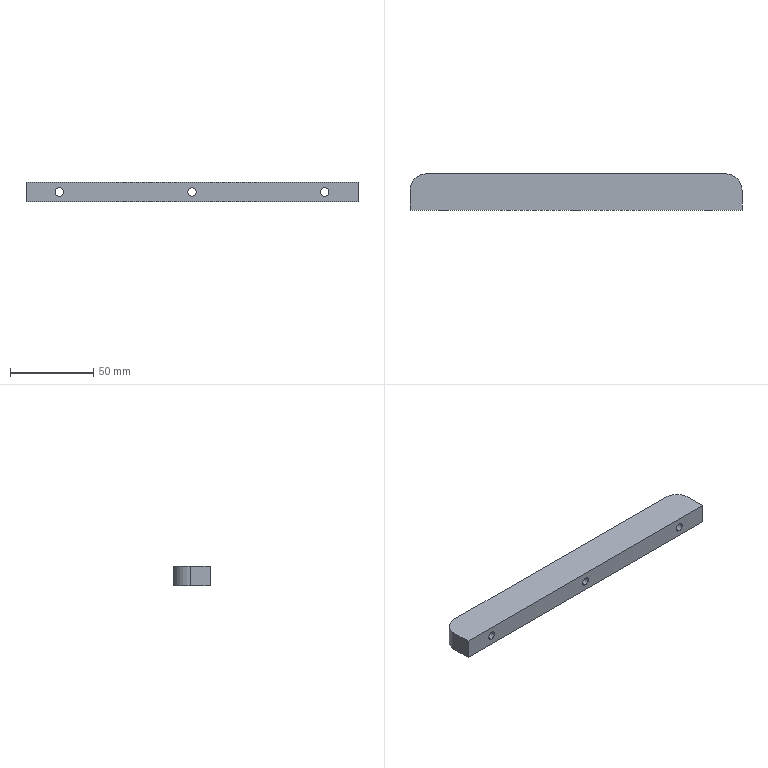Part | STEP file | 02-Support strip | 1 solid | 14 faces | box 200 x 22 x 12 mm | volume 50989 mm3 | cylinder 8 | plane 6 | commonest cylinder face diameters 5 x6 20 x2
STEP:
#1=CARTESIAN_POINT('',(0.,0.,0.));
#2=DIRECTION('',(0.,0.,1.));
#3=DIRECTION('',(1.,0.,0.));
#4=AXIS2_PLACEMENT_3D('',#1,#2,#3);
#5=CARTESIAN_POINT('',(180.,0.,8.5));
#6=VERTEX_POINT('',#5);
#7=CARTESIAN_POINT('',(180.,22.,8.5));
#8=VERTEX_POINT('',#7);
#9=CARTESIAN_POINT('',(180.,22.,8.5));
#10=DIRECTION('',(0.,1.,0.));
#11=VECTOR('',#10,1.);
#12=LINE('',#9,#11);
#13=CARTESIAN_POINT('',(180.,22.,6.));
#14=DIRECTION('',(0.,1.,0.));
#15=DIRECTION('',(0.,0.,1.));
#16=AXIS2_PLACEMENT_3D('',#13,#14,#15);
#17=CYLINDRICAL_SURFACE('',#16,2.5);
#18=CARTESIAN_POINT('',(6.283,0.));
#19=DIRECTION('',(0.,1.));
#20=VECTOR('',#19,1.);
#21=LINE('',#18,#20);
#22=(GEOMETRIC_REPRESENTATION_CONTEXT(2)PARAMETRIC_REPRESENTATION_CONTEXT()REPRESENTATION_CONTEXT('',''));
#23=DEFINITIONAL_REPRESENTATION('',(#21),#22);
#24=PCURVE('',#17,#23);
#25=CARTESIAN_POINT('',(180.,22.,6.));
#26=DIRECTION('',(0.,1.,0.));
#27=DIRECTION('',(0.,0.,1.));
#28=AXIS2_PLACEMENT_3D('',#25,#26,#27);
#29=CYLINDRICAL_SURFACE('',#28,2.5);
#30=CARTESIAN_POINT('',(0.,0.));
#31=DIRECTION('',(0.,1.));
#32=VECTOR('',#31,1.);
#33=LINE('',#30,#32);
#34=(GEOMETRIC_REPRESENTATION_CONTEXT(2)PARAMETRIC_REPRESENTATION_CONTEXT()REPRESENTATION_CONTEXT('',''));
#35=DEFINITIONAL_REPRESENTATION('',(#33),#34);
#36=PCURVE('',#29,#35);
#37=SURFACE_CURVE('',#12,(#24,#36),.PCURVE_S1.);
#38=EDGE_CURVE('',#6,#8,#37,.T.);
#39=ORIENTED_EDGE('',*,*,#38,.T.);
#40=CARTESIAN_POINT('',(180.,22.,3.5));
#41=VERTEX_POINT('',#40);
#42=CARTESIAN_POINT('',(180.,22.,6.));
#43=DIRECTION('',(0.,1.,0.));
#44=DIRECTION('',(0.,0.,1.));
#45=AXIS2_PLACEMENT_3D('',#42,#43,#44);
#46=CIRCLE('',#45,2.5);
#47=CARTESIAN_POINT('',(0.,0.));
#48=DIRECTION('',(1.,0.));
#49=VECTOR('',#48,1.);
#50=LINE('',#47,#49);
#51=(GEOMETRIC_REPRESENTATION_CONTEXT(2)PARAMETRIC_REPRESENTATION_CONTEXT()REPRESENTATION_CONTEXT('',''));
#52=DEFINITIONAL_REPRESENTATION('',(#50),#51);
#53=PCURVE('',#17,#52);
#54=CARTESIAN_POINT('',(10.,22.,12.));
#55=DIRECTION('',(0.,-1.,0.));
#56=DIRECTION('',(0.,0.,-1.));
#57=AXIS2_PLACEMENT_3D('',#54,#55,#56);
#58=PLANE('',#57);
#59=CARTESIAN_POINT('',(3.5,170.));
#60=CARTESIAN_POINT('',(3.5,174.33));
#61=CARTESIAN_POINT('',(7.25,172.165));
#62=CARTESIAN_POINT('',(11.,170.));
#63=CARTESIAN_POINT('',(7.25,167.835));
#64=CARTESIAN_POINT('',(3.5,165.67));
#65=CARTESIAN_POINT('',(3.5,170.));
#66=(BOUNDED_CURVE()B_SPLINE_CURVE(2,(#59,#60,#61,#62,#63,#64,#65),.UNSPECIFIED.,.T.,.F.)B_SPLINE_CURVE_WITH_KNOTS((1,2,2,2,2,1),(-2.094,0.,2.094,4.189,6.283,8.378),.UNSPECIFIED.)CURVE()GEOMETRIC_REPRESENTATION_ITEM()RATIONAL_B_SPLINE_CURVE((1.,0.5,1.,0.5,1.,0.5,1.))REPRESENTATION_ITEM(''));
#67=(GEOMETRIC_REPRESENTATION_CONTEXT(2)PARAMETRIC_REPRESENTATION_CONTEXT()REPRESENTATION_CONTEXT('',''));
#68=DEFINITIONAL_REPRESENTATION('',(#66),#67);
#69=PCURVE('',#58,#68);
#70=SURFACE_CURVE('',#46,(#53,#69),.PCURVE_S1.);
#71=EDGE_CURVE('',#41,#8,#70,.T.);
#72=ORIENTED_EDGE('',*,*,#71,.F.);
#73=CARTESIAN_POINT('',(180.,0.,3.5));
#74=VERTEX_POINT('',#73);
#75=CARTESIAN_POINT('',(180.,22.,3.5));
#76=DIRECTION('',(0.,1.,0.));
#77=VECTOR('',#76,1.);
#78=LINE('',#75,#77);
#79=CARTESIAN_POINT('',(3.142,0.));
#80=DIRECTION('',(0.,1.));
#81=VECTOR('',#80,1.);
#82=LINE('',#79,#81);
#83=(GEOMETRIC_REPRESENTATION_CONTEXT(2)PARAMETRIC_REPRESENTATION_CONTEXT()REPRESENTATION_CONTEXT('',''));
#84=DEFINITIONAL_REPRESENTATION('',(#82),#83);
#85=PCURVE('',#17,#84);
#86=CARTESIAN_POINT('',(3.142,0.));
#87=DIRECTION('',(0.,1.));
#88=VECTOR('',#87,1.);
#89=LINE('',#86,#88);
#90=(GEOMETRIC_REPRESENTATION_CONTEXT(2)PARAMETRIC_REPRESENTATION_CONTEXT()REPRESENTATION_CONTEXT('',''));
#91=DEFINITIONAL_REPRESENTATION('',(#89),#90);
#92=PCURVE('',#29,#91);
#93=SURFACE_CURVE('',#78,(#85,#92),.PCURVE_S1.);
#94=EDGE_CURVE('',#74,#41,#93,.T.);
#95=ORIENTED_EDGE('',*,*,#94,.F.);
#96=CARTESIAN_POINT('',(180.,0.,6.));
#97=DIRECTION('',(0.,1.,0.));
#98=DIRECTION('',(0.,0.,1.));
#99=AXIS2_PLACEMENT_3D('',#96,#97,#98);
#100=CIRCLE('',#99,2.5);
#101=CARTESIAN_POINT('',(0.,-22.));
#102=DIRECTION('',(1.,0.));
#103=VECTOR('',#102,1.);
#104=LINE('',#101,#103);
#105=(GEOMETRIC_REPRESENTATION_CONTEXT(2)PARAMETRIC_REPRESENTATION_CONTEXT()REPRESENTATION_CONTEXT('',''));
#106=DEFINITIONAL_REPRESENTATION('',(#104),#105);
#107=PCURVE('',#17,#106);
#108=CARTESIAN_POINT('',(0.,0.,12.));
#109=DIRECTION('',(0.,1.,0.));
#110=DIRECTION('',(0.,0.,1.));
#111=AXIS2_PLACEMENT_3D('',#108,#109,#110);
#112=PLANE('',#111);
#113=CARTESIAN_POINT('',(-6.,180.));
#114=DIRECTION('',(1.,0.));
#115=AXIS2_PLACEMENT_2D('',#113,#114);
#116=CIRCLE('',#115,2.5);
#117=(GEOMETRIC_REPRESENTATION_CONTEXT(2)PARAMETRIC_REPRESENTATION_CONTEXT()REPRESENTATION_CONTEXT('',''));
#118=DEFINITIONAL_REPRESENTATION('',(#116),#117);
#119=PCURVE('',#112,#118);
#120=SURFACE_CURVE('',#100,(#107,#119),.PCURVE_S1.);
#121=EDGE_CURVE('',#74,#6,#120,.T.);
#122=ORIENTED_EDGE('',*,*,#121,.T.);
#123=EDGE_LOOP('',(#39,#72,#95,#122));
#124=FACE_BOUND('',#123,.F.);
#125=ADVANCED_FACE('',(#124),#17,.F.);
#126=CARTESIAN_POINT('',(100.,0.,8.5));
#127=VERTEX_POINT('',#126);
#128=CARTESIAN_POINT('',(100.,22.,8.5));
#129=VERTEX_POINT('',#128);
#130=CARTESIAN_POINT('',(100.,22.,8.5));
#131=DIRECTION('',(0.,1.,0.));
#132=VECTOR('',#131,1.);
#133=LINE('',#130,#132);
#134=CARTESIAN_POINT('',(100.,22.,6.));
#135=DIRECTION('',(0.,1.,0.));
#136=DIRECTION('',(0.,0.,1.));
#137=AXIS2_PLACEMENT_3D('',#134,#135,#136);
#138=CYLINDRICAL_SURFACE('',#137,2.5);
#139=CARTESIAN_POINT('',(6.283,0.));
#140=DIRECTION('',(0.,1.));
#141=VECTOR('',#140,1.);
#142=LINE('',#139,#141);
#143=(GEOMETRIC_REPRESENTATION_CONTEXT(2)PARAMETRIC_REPRESENTATION_CONTEXT()REPRESENTATION_CONTEXT('',''));
#144=DEFINITIONAL_REPRESENTATION('',(#142),#143);
#145=PCURVE('',#138,#144);
#146=CARTESIAN_POINT('',(100.,22.,6.));
#147=DIRECTION('',(0.,1.,0.));
#148=DIRECTION('',(0.,0.,1.));
#149=AXIS2_PLACEMENT_3D('',#146,#147,#148);
#150=CYLINDRICAL_SURFACE('',#149,2.5);
#151=CARTESIAN_POINT('',(0.,0.));
#152=DIRECTION('',(0.,1.));
#153=VECTOR('',#152,1.);
#154=LINE('',#151,#153);
#155=(GEOMETRIC_REPRESENTATION_CONTEXT(2)PARAMETRIC_REPRESENTATION_CONTEXT()REPRESENTATION_CONTEXT('',''));
#156=DEFINITIONAL_REPRESENTATION('',(#154),#155);
#157=PCURVE('',#150,#156);
#158=SURFACE_CURVE('',#133,(#145,#157),.PCURVE_S1.);
#159=EDGE_CURVE('',#127,#129,#158,.T.);
#160=ORIENTED_EDGE('',*,*,#159,.T.);
#161=CARTESIAN_POINT('',(100.,22.,3.5));
#162=VERTEX_POINT('',#161);
#163=CARTESIAN_POINT('',(100.,22.,6.));
#164=DIRECTION('',(0.,1.,0.));
#165=DIRECTION('',(0.,0.,1.));
#166=AXIS2_PLACEMENT_3D('',#163,#164,#165);
#167=CIRCLE('',#166,2.5);
#168=CARTESIAN_POINT('',(0.,0.));
#169=DIRECTION('',(1.,0.));
#170=VECTOR('',#169,1.);
#171=LINE('',#168,#170);
#172=(GEOMETRIC_REPRESENTATION_CONTEXT(2)PARAMETRIC_REPRESENTATION_CONTEXT()REPRESENTATION_CONTEXT('',''));
#173=DEFINITIONAL_REPRESENTATION('',(#171),#172);
#174=PCURVE('',#138,#173);
#175=CARTESIAN_POINT('',(3.5,90.));
#176=CARTESIAN_POINT('',(3.5,94.33));
#177=CARTESIAN_POINT('',(7.25,92.165));
#178=CARTESIAN_POINT('',(11.,90.));
#179=CARTESIAN_POINT('',(7.25,87.835));
#180=CARTESIAN_POINT('',(3.5,85.67));
#181=CARTESIAN_POINT('',(3.5,90.));
#182=(BOUNDED_CURVE()B_SPLINE_CURVE(2,(#175,#176,#177,#178,#179,#180,#181),.UNSPECIFIED.,.T.,.F.)B_SPLINE_CURVE_WITH_KNOTS((1,2,2,2,2,1),(-2.094,0.,2.094,4.189,6.283,8.378),.UNSPECIFIED.)CURVE()GEOMETRIC_REPRESENTATION_ITEM()RATIONAL_B_SPLINE_CURVE((1.,0.5,1.,0.5,1.,0.5,1.))REPRESENTATION_ITEM(''));
#183=(GEOMETRIC_REPRESENTATION_CONTEXT(2)PARAMETRIC_REPRESENTATION_CONTEXT()REPRESENTATION_CONTEXT('',''));
#184=DEFINITIONAL_REPRESENTATION('',(#182),#183);
#185=PCURVE('',#58,#184);
#186=SURFACE_CURVE('',#167,(#174,#185),.PCURVE_S1.);
#187=EDGE_CURVE('',#162,#129,#186,.T.);
#188=ORIENTED_EDGE('',*,*,#187,.F.);
#189=CARTESIAN_POINT('',(100.,0.,3.5));
#190=VERTEX_POINT('',#189);
#191=CARTESIAN_POINT('',(100.,22.,3.5));
#192=DIRECTION('',(0.,1.,0.));
#193=VECTOR('',#192,1.);
#194=LINE('',#191,#193);
#195=CARTESIAN_POINT('',(3.142,0.));
#196=DIRECTION('',(0.,1.));
#197=VECTOR('',#196,1.);
#198=LINE('',#195,#197);
#199=(GEOMETRIC_REPRESENTATION_CONTEXT(2)PARAMETRIC_REPRESENTATION_CONTEXT()REPRESENTATION_CONTEXT('',''));
#200=DEFINITIONAL_REPRESENTATION('',(#198),#199);
#201=PCURVE('',#138,#200);
#202=CARTESIAN_POINT('',(3.142,0.));
#203=DIRECTION('',(0.,1.));
#204=VECTOR('',#203,1.);
#205=LINE('',#202,#204);
#206=(GEOMETRIC_REPRESENTATION_CONTEXT(2)PARAMETRIC_REPRESENTATION_CONTEXT()REPRESENTATION_CONTEXT('',''));
#207=DEFINITIONAL_REPRESENTATION('',(#205),#206);
#208=PCURVE('',#150,#207);
#209=SURFACE_CURVE('',#194,(#201,#208),.PCURVE_S1.);
#210=EDGE_CURVE('',#190,#162,#209,.T.);
#211=ORIENTED_EDGE('',*,*,#210,.F.);
#212=CARTESIAN_POINT('',(100.,0.,6.));
#213=DIRECTION('',(0.,1.,0.));
#214=DIRECTION('',(0.,0.,1.));
#215=AXIS2_PLACEMENT_3D('',#212,#213,#214);
#216=CIRCLE('',#215,2.5);
#217=CARTESIAN_POINT('',(0.,-22.));
#218=DIRECTION('',(1.,0.));
#219=VECTOR('',#218,1.);
#220=LINE('',#217,#219);
#221=(GEOMETRIC_REPRESENTATION_CONTEXT(2)PARAMETRIC_REPRESENTATION_CONTEXT()REPRESENTATION_CONTEXT('',''));
#222=DEFINITIONAL_REPRESENTATION('',(#220),#221);
#223=PCURVE('',#138,#222);
#224=CARTESIAN_POINT('',(-6.,100.));
#225=DIRECTION('',(1.,0.));
#226=AXIS2_PLACEMENT_2D('',#224,#225);
#227=CIRCLE('',#226,2.5);
#228=(GEOMETRIC_REPRESENTATION_CONTEXT(2)PARAMETRIC_REPRESENTATION_CONTEXT()REPRESENTATION_CONTEXT('',''));
#229=DEFINITIONAL_REPRESENTATION('',(#227),#228);
#230=PCURVE('',#112,#229);
#231=SURFACE_CURVE('',#216,(#223,#230),.PCURVE_S1.);
#232=EDGE_CURVE('',#190,#127,#231,.T.);
#233=ORIENTED_EDGE('',*,*,#232,.T.);
#234=EDGE_LOOP('',(#160,#188,#211,#233));
#235=FACE_BOUND('',#234,.F.);
#236=ADVANCED_FACE('',(#235),#138,.F.);
#237=CARTESIAN_POINT('',(20.,0.,8.5));
#238=VERTEX_POINT('',#237);
#239=CARTESIAN_POINT('',(20.,22.,8.5));
#240=VERTEX_POINT('',#239);
#241=CARTESIAN_POINT('',(20.,22.,8.5));
#242=DIRECTION('',(0.,1.,0.));
#243=VECTOR('',#242,1.);
#244=LINE('',#241,#243);
#245=CARTESIAN_POINT('',(20.,22.,6.));
#246=DIRECTION('',(0.,1.,0.));
#247=DIRECTION('',(0.,0.,1.));
#248=AXIS2_PLACEMENT_3D('',#245,#246,#247);
#249=CYLINDRICAL_SURFACE('',#248,2.5);
#250=CARTESIAN_POINT('',(6.283,0.));
#251=DIRECTION('',(0.,1.));
#252=VECTOR('',#251,1.);
#253=LINE('',#250,#252);
#254=(GEOMETRIC_REPRESENTATION_CONTEXT(2)PARAMETRIC_REPRESENTATION_CONTEXT()REPRESENTATION_CONTEXT('',''));
#255=DEFINITIONAL_REPRESENTATION('',(#253),#254);
#256=PCURVE('',#249,#255);
#257=CARTESIAN_POINT('',(20.,22.,6.));
#258=DIRECTION('',(0.,1.,0.));
#259=DIRECTION('',(0.,0.,1.));
#260=AXIS2_PLACEMENT_3D('',#257,#258,#259);
#261=CYLINDRICAL_SURFACE('',#260,2.5);
#262=CARTESIAN_POINT('',(0.,0.));
#263=DIRECTION('',(0.,1.));
#264=VECTOR('',#263,1.);
#265=LINE('',#262,#264);
#266=(GEOMETRIC_REPRESENTATION_CONTEXT(2)PARAMETRIC_REPRESENTATION_CONTEXT()REPRESENTATION_CONTEXT('',''));
#267=DEFINITIONAL_REPRESENTATION('',(#265),#266);
#268=PCURVE('',#261,#267);
#269=SURFACE_CURVE('',#244,(#256,#268),.PCURVE_S1.);
#270=EDGE_CURVE('',#238,#240,#269,.T.);
#271=ORIENTED_EDGE('',*,*,#270,.T.);
#272=CARTESIAN_POINT('',(20.,22.,3.5));
#273=VERTEX_POINT('',#272);
#274=CARTESIAN_POINT('',(20.,22.,6.));
#275=DIRECTION('',(0.,1.,0.));
#276=DIRECTION('',(0.,0.,1.));
#277=AXIS2_PLACEMENT_3D('',#274,#275,#276);
#278=CIRCLE('',#277,2.5);
#279=CARTESIAN_POINT('',(0.,0.));
#280=DIRECTION('',(1.,0.));
#281=VECTOR('',#280,1.);
#282=LINE('',#279,#281);
#283=(GEOMETRIC_REPRESENTATION_CONTEXT(2)PARAMETRIC_REPRESENTATION_CONTEXT()REPRESENTATION_CONTEXT('',''));
#284=DEFINITIONAL_REPRESENTATION('',(#282),#283);
#285=PCURVE('',#249,#284);
#286=CARTESIAN_POINT('',(3.5,10.));
#287=CARTESIAN_POINT('',(3.5,14.33));
#288=CARTESIAN_POINT('',(7.25,12.165));
#289=CARTESIAN_POINT('',(11.,10.));
#290=CARTESIAN_POINT('',(7.25,7.835));
#291=CARTESIAN_POINT('',(3.5,5.67));
#292=CARTESIAN_POINT('',(3.5,10.));
#293=(BOUNDED_CURVE()B_SPLINE_CURVE(2,(#286,#287,#288,#289,#290,#291,#292),.UNSPECIFIED.,.T.,.F.)B_SPLINE_CURVE_WITH_KNOTS((1,2,2,2,2,1),(-2.094,0.,2.094,4.189,6.283,8.378),.UNSPECIFIED.)CURVE()GEOMETRIC_REPRESENTATION_ITEM()RATIONAL_B_SPLINE_CURVE((1.,0.5,1.,0.5,1.,0.5,1.))REPRESENTATION_ITEM(''));
#294=(GEOMETRIC_REPRESENTATION_CONTEXT(2)PARAMETRIC_REPRESENTATION_CONTEXT()REPRESENTATION_CONTEXT('',''));
#295=DEFINITIONAL_REPRESENTATION('',(#293),#294);
#296=PCURVE('',#58,#295);
#297=SURFACE_CURVE('',#278,(#285,#296),.PCURVE_S1.);
#298=EDGE_CURVE('',#273,#240,#297,.T.);
#299=ORIENTED_EDGE('',*,*,#298,.F.);
#300=CARTESIAN_POINT('',(20.,0.,3.5));
#301=VERTEX_POINT('',#300);
#302=CARTESIAN_POINT('',(20.,22.,3.5));
#303=DIRECTION('',(0.,1.,0.));
#304=VECTOR('',#303,1.);
#305=LINE('',#302,#304);
#306=CARTESIAN_POINT('',(3.142,0.));
#307=DIRECTION('',(0.,1.));
#308=VECTOR('',#307,1.);
#309=LINE('',#306,#308);
#310=(GEOMETRIC_REPRESENTATION_CONTEXT(2)PARAMETRIC_REPRESENTATION_CONTEXT()REPRESENTATION_CONTEXT('',''));
#311=DEFINITIONAL_REPRESENTATION('',(#309),#310);
#312=PCURVE('',#249,#311);
#313=CARTESIAN_POINT('',(3.142,0.));
#314=DIRECTION('',(0.,1.));
#315=VECTOR('',#314,1.);
#316=LINE('',#313,#315);
#317=(GEOMETRIC_REPRESENTATION_CONTEXT(2)PARAMETRIC_REPRESENTATION_CONTEXT()REPRESENTATION_CONTEXT('',''));
#318=DEFINITIONAL_REPRESENTATION('',(#316),#317);
#319=PCURVE('',#261,#318);
#320=SURFACE_CURVE('',#305,(#312,#319),.PCURVE_S1.);
#321=EDGE_CURVE('',#301,#273,#320,.T.);
#322=ORIENTED_EDGE('',*,*,#321,.F.);
#323=CARTESIAN_POINT('',(20.,0.,6.));
#324=DIRECTION('',(0.,1.,0.));
#325=DIRECTION('',(0.,0.,1.));
#326=AXIS2_PLACEMENT_3D('',#323,#324,#325);
#327=CIRCLE('',#326,2.5);
#328=CARTESIAN_POINT('',(0.,-22.));
#329=DIRECTION('',(1.,0.));
#330=VECTOR('',#329,1.);
#331=LINE('',#328,#330);
#332=(GEOMETRIC_REPRESENTATION_CONTEXT(2)PARAMETRIC_REPRESENTATION_CONTEXT()REPRESENTATION_CONTEXT('',''));
#333=DEFINITIONAL_REPRESENTATION('',(#331),#332);
#334=PCURVE('',#249,#333);
#335=CARTESIAN_POINT('',(-6.,20.));
#336=DIRECTION('',(1.,0.));
#337=AXIS2_PLACEMENT_2D('',#335,#336);
#338=CIRCLE('',#337,2.5);
#339=(GEOMETRIC_REPRESENTATION_CONTEXT(2)PARAMETRIC_REPRESENTATION_CONTEXT()REPRESENTATION_CONTEXT('',''));
#340=DEFINITIONAL_REPRESENTATION('',(#338),#339);
#341=PCURVE('',#112,#340);
#342=SURFACE_CURVE('',#327,(#334,#341),.PCURVE_S1.);
#343=EDGE_CURVE('',#301,#238,#342,.T.);
#344=ORIENTED_EDGE('',*,*,#343,.T.);
#345=EDGE_LOOP('',(#271,#299,#322,#344));
#346=FACE_BOUND('',#345,.F.);
#347=ADVANCED_FACE('',(#346),#249,.F.);
#348=CARTESIAN_POINT('',(0.,12.,0.));
#349=VERTEX_POINT('',#348);
#350=CARTESIAN_POINT('',(0.,0.,0.));
#351=VERTEX_POINT('',#350);
#352=CARTESIAN_POINT('',(0.,0.,0.));
#353=DIRECTION('',(0.,-1.,0.));
#354=VECTOR('',#353,1.);
#355=LINE('',#352,#354);
#356=CARTESIAN_POINT('',(0.,0.,12.));
#357=DIRECTION('',(1.,0.,0.));
#358=DIRECTION('',(0.,0.,-1.));
#359=AXIS2_PLACEMENT_3D('',#356,#357,#358);
#360=PLANE('',#359);
#361=CARTESIAN_POINT('',(12.,0.));
#362=DIRECTION('',(0.,-1.));
#363=VECTOR('',#362,1.);
#364=LINE('',#361,#363);
#365=(GEOMETRIC_REPRESENTATION_CONTEXT(2)PARAMETRIC_REPRESENTATION_CONTEXT()REPRESENTATION_CONTEXT('',''));
#366=DEFINITIONAL_REPRESENTATION('',(#364),#365);
#367=PCURVE('',#360,#366);
#368=CARTESIAN_POINT('',(10.,12.,0.));
#369=DIRECTION('',(0.,0.,-1.));
#370=DIRECTION('',(-1.,0.,0.));
#371=AXIS2_PLACEMENT_3D('',#368,#369,#370);
#372=PLANE('',#371);
#373=CARTESIAN_POINT('',(10.,-12.));
#374=DIRECTION('',(0.,-1.));
#375=VECTOR('',#374,1.);
#376=LINE('',#373,#375);
#377=(GEOMETRIC_REPRESENTATION_CONTEXT(2)PARAMETRIC_REPRESENTATION_CONTEXT()REPRESENTATION_CONTEXT('',''));
#378=DEFINITIONAL_REPRESENTATION('',(#376),#377);
#379=PCURVE('',#372,#378);
#380=SURFACE_CURVE('',#355,(#367,#379),.PCURVE_S1.);
#381=EDGE_CURVE('',#349,#351,#380,.T.);
#382=ORIENTED_EDGE('',*,*,#381,.T.);
#383=CARTESIAN_POINT('',(0.,0.,12.));
#384=VERTEX_POINT('',#383);
#385=CARTESIAN_POINT('',(0.,0.,12.));
#386=DIRECTION('',(0.,0.,-1.));
#387=VECTOR('',#386,1.);
#388=LINE('',#385,#387);
#389=CARTESIAN_POINT('',(0.,0.));
#390=DIRECTION('',(1.,0.));
#391=VECTOR('',#390,1.);
#392=LINE('',#389,#391);
#393=(GEOMETRIC_REPRESENTATION_CONTEXT(2)PARAMETRIC_REPRESENTATION_CONTEXT()REPRESENTATION_CONTEXT('',''));
#394=DEFINITIONAL_REPRESENTATION('',(#392),#393);
#395=PCURVE('',#360,#394);
#396=CARTESIAN_POINT('',(0.,0.));
#397=DIRECTION('',(-1.,0.));
#398=VECTOR('',#397,1.);
#399=LINE('',#396,#398);
#400=(GEOMETRIC_REPRESENTATION_CONTEXT(2)PARAMETRIC_REPRESENTATION_CONTEXT()REPRESENTATION_CONTEXT('',''));
#401=DEFINITIONAL_REPRESENTATION('',(#399),#400);
#402=PCURVE('',#112,#401);
#403=SURFACE_CURVE('',#388,(#395,#402),.PCURVE_S1.);
#404=EDGE_CURVE('',#384,#351,#403,.T.);
#405=ORIENTED_EDGE('',*,*,#404,.F.);
#406=CARTESIAN_POINT('',(0.,12.,12.));
#407=VERTEX_POINT('',#406);
#408=CARTESIAN_POINT('',(0.,0.,12.));
#409=DIRECTION('',(0.,-1.,0.));
#410=VECTOR('',#409,1.);
#411=LINE('',#408,#410);
#412=CARTESIAN_POINT('',(0.,0.));
#413=DIRECTION('',(0.,-1.));
#414=VECTOR('',#413,1.);
#415=LINE('',#412,#414);
#416=(GEOMETRIC_REPRESENTATION_CONTEXT(2)PARAMETRIC_REPRESENTATION_CONTEXT()REPRESENTATION_CONTEXT('',''));
#417=DEFINITIONAL_REPRESENTATION('',(#415),#416);
#418=PCURVE('',#360,#417);
#419=CARTESIAN_POINT('',(10.,12.,12.));
#420=DIRECTION('',(0.,0.,-1.));
#421=DIRECTION('',(-1.,0.,0.));
#422=AXIS2_PLACEMENT_3D('',#419,#420,#421);
#423=PLANE('',#422);
#424=CARTESIAN_POINT('',(10.,-12.));
#425=DIRECTION('',(0.,-1.));
#426=VECTOR('',#425,1.);
#427=LINE('',#424,#426);
#428=(GEOMETRIC_REPRESENTATION_CONTEXT(2)PARAMETRIC_REPRESENTATION_CONTEXT()REPRESENTATION_CONTEXT('',''));
#429=DEFINITIONAL_REPRESENTATION('',(#427),#428);
#430=PCURVE('',#423,#429);
#431=SURFACE_CURVE('',#411,(#418,#430),.PCURVE_S1.);
#432=EDGE_CURVE('',#407,#384,#431,.T.);
#433=ORIENTED_EDGE('',*,*,#432,.F.);
#434=CARTESIAN_POINT('',(0.,12.,12.));
#435=DIRECTION('',(0.,0.,-1.));
#436=VECTOR('',#435,1.);
#437=LINE('',#434,#436);
#438=CARTESIAN_POINT('',(0.,12.));
#439=DIRECTION('',(1.,0.));
#440=VECTOR('',#439,1.);
#441=LINE('',#438,#440);
#442=(GEOMETRIC_REPRESENTATION_CONTEXT(2)PARAMETRIC_REPRESENTATION_CONTEXT()REPRESENTATION_CONTEXT('',''));
#443=DEFINITIONAL_REPRESENTATION('',(#441),#442);
#444=PCURVE('',#360,#443);
#445=CARTESIAN_POINT('',(10.,12.,12.));
#446=DIRECTION('',(0.,0.,-1.));
#447=DIRECTION('',(-1.,0.,0.));
#448=AXIS2_PLACEMENT_3D('',#445,#446,#447);
#449=CYLINDRICAL_SURFACE('',#448,10.);
#450=CARTESIAN_POINT('',(0.,0.));
#451=DIRECTION('',(0.,1.));
#452=VECTOR('',#451,1.);
#453=LINE('',#450,#452);
#454=(GEOMETRIC_REPRESENTATION_CONTEXT(2)PARAMETRIC_REPRESENTATION_CONTEXT()REPRESENTATION_CONTEXT('',''));
#455=DEFINITIONAL_REPRESENTATION('',(#453),#454);
#456=PCURVE('',#449,#455);
#457=SURFACE_CURVE('',#437,(#444,#456),.PCURVE_S1.);
#458=EDGE_CURVE('',#407,#349,#457,.T.);
#459=ORIENTED_EDGE('',*,*,#458,.T.);
#460=EDGE_LOOP('',(#382,#405,#433,#459));
#461=FACE_BOUND('',#460,.T.);
#462=ADVANCED_FACE('',(#461),#360,.F.);
#463=CARTESIAN_POINT('',(180.,0.,6.));
#464=DIRECTION('',(0.,1.,0.));
#465=DIRECTION('',(0.,0.,1.));
#466=AXIS2_PLACEMENT_3D('',#463,#464,#465);
#467=CIRCLE('',#466,2.5);
#468=CARTESIAN_POINT('',(-6.,180.));
#469=DIRECTION('',(1.,0.));
#470=AXIS2_PLACEMENT_2D('',#468,#469);
#471=CIRCLE('',#470,2.5);
#472=(GEOMETRIC_REPRESENTATION_CONTEXT(2)PARAMETRIC_REPRESENTATION_CONTEXT()REPRESENTATION_CONTEXT('',''));
#473=DEFINITIONAL_REPRESENTATION('',(#471),#472);
#474=PCURVE('',#112,#473);
#475=CARTESIAN_POINT('',(0.,-22.));
#476=DIRECTION('',(1.,0.));
#477=VECTOR('',#476,1.);
#478=LINE('',#475,#477);
#479=(GEOMETRIC_REPRESENTATION_CONTEXT(2)PARAMETRIC_REPRESENTATION_CONTEXT()REPRESENTATION_CONTEXT('',''));
#480=DEFINITIONAL_REPRESENTATION('',(#478),#479);
#481=PCURVE('',#29,#480);
#482=SURFACE_CURVE('',#467,(#474,#481),.PCURVE_S1.);
#483=EDGE_CURVE('',#6,#74,#482,.T.);
#484=ORIENTED_EDGE('',*,*,#483,.T.);
#485=ORIENTED_EDGE('',*,*,#121,.T.);
#486=EDGE_LOOP('',(#484,#485));
#487=FACE_BOUND('',#486,.T.);
#488=CARTESIAN_POINT('',(100.,0.,6.));
#489=DIRECTION('',(0.,1.,0.));
#490=DIRECTION('',(0.,0.,1.));
#491=AXIS2_PLACEMENT_3D('',#488,#489,#490);
#492=CIRCLE('',#491,2.5);
#493=CARTESIAN_POINT('',(-6.,100.));
#494=DIRECTION('',(1.,0.));
#495=AXIS2_PLACEMENT_2D('',#493,#494);
#496=CIRCLE('',#495,2.5);
#497=(GEOMETRIC_REPRESENTATION_CONTEXT(2)PARAMETRIC_REPRESENTATION_CONTEXT()REPRESENTATION_CONTEXT('',''));
#498=DEFINITIONAL_REPRESENTATION('',(#496),#497);
#499=PCURVE('',#112,#498);
#500=CARTESIAN_POINT('',(0.,-22.));
#501=DIRECTION('',(1.,0.));
#502=VECTOR('',#501,1.);
#503=LINE('',#500,#502);
#504=(GEOMETRIC_REPRESENTATION_CONTEXT(2)PARAMETRIC_REPRESENTATION_CONTEXT()REPRESENTATION_CONTEXT('',''));
#505=DEFINITIONAL_REPRESENTATION('',(#503),#504);
#506=PCURVE('',#150,#505);
#507=SURFACE_CURVE('',#492,(#499,#506),.PCURVE_S1.);
#508=EDGE_CURVE('',#127,#190,#507,.T.);
#509=ORIENTED_EDGE('',*,*,#508,.T.);
#510=ORIENTED_EDGE('',*,*,#232,.T.);
#511=EDGE_LOOP('',(#509,#510));
#512=FACE_BOUND('',#511,.T.);
#513=CARTESIAN_POINT('',(20.,0.,6.));
#514=DIRECTION('',(0.,1.,0.));
#515=DIRECTION('',(0.,0.,1.));
#516=AXIS2_PLACEMENT_3D('',#513,#514,#515);
#517=CIRCLE('',#516,2.5);
#518=CARTESIAN_POINT('',(-6.,20.));
#519=DIRECTION('',(1.,0.));
#520=AXIS2_PLACEMENT_2D('',#518,#519);
#521=CIRCLE('',#520,2.5);
#522=(GEOMETRIC_REPRESENTATION_CONTEXT(2)PARAMETRIC_REPRESENTATION_CONTEXT()REPRESENTATION_CONTEXT('',''));
#523=DEFINITIONAL_REPRESENTATION('',(#521),#522);
#524=PCURVE('',#112,#523);
#525=CARTESIAN_POINT('',(0.,-22.));
#526=DIRECTION('',(1.,0.));
#527=VECTOR('',#526,1.);
#528=LINE('',#525,#527);
#529=(GEOMETRIC_REPRESENTATION_CONTEXT(2)PARAMETRIC_REPRESENTATION_CONTEXT()REPRESENTATION_CONTEXT('',''));
#530=DEFINITIONAL_REPRESENTATION('',(#528),#529);
#531=PCURVE('',#261,#530);
#532=SURFACE_CURVE('',#517,(#524,#531),.PCURVE_S1.);
#533=EDGE_CURVE('',#238,#301,#532,.T.);
#534=ORIENTED_EDGE('',*,*,#533,.T.);
#535=ORIENTED_EDGE('',*,*,#343,.T.);
#536=EDGE_LOOP('',(#534,#535));
#537=FACE_BOUND('',#536,.T.);
#538=CARTESIAN_POINT('',(200.,0.,0.));
#539=VERTEX_POINT('',#538);
#540=CARTESIAN_POINT('',(0.,0.,0.));
#541=DIRECTION('',(1.,0.,0.));
#542=VECTOR('',#541,1.);
#543=LINE('',#540,#542);
#544=CARTESIAN_POINT('',(-12.,0.));
#545=DIRECTION('',(0.,1.));
#546=VECTOR('',#545,1.);
#547=LINE('',#544,#546);
#548=(GEOMETRIC_REPRESENTATION_CONTEXT(2)PARAMETRIC_REPRESENTATION_CONTEXT()REPRESENTATION_CONTEXT('',''));
#549=DEFINITIONAL_REPRESENTATION('',(#547),#548);
#550=PCURVE('',#112,#549);
#551=CARTESIAN_POINT('',(10.,-12.));
#552=DIRECTION('',(-1.,0.));
#553=VECTOR('',#552,1.);
#554=LINE('',#551,#553);
#555=(GEOMETRIC_REPRESENTATION_CONTEXT(2)PARAMETRIC_REPRESENTATION_CONTEXT()REPRESENTATION_CONTEXT('',''));
#556=DEFINITIONAL_REPRESENTATION('',(#554),#555);
#557=PCURVE('',#372,#556);
#558=SURFACE_CURVE('',#543,(#550,#557),.PCURVE_S1.);
#559=EDGE_CURVE('',#351,#539,#558,.T.);
#560=ORIENTED_EDGE('',*,*,#559,.T.);
#561=CARTESIAN_POINT('',(200.,0.,12.));
#562=VERTEX_POINT('',#561);
#563=CARTESIAN_POINT('',(200.,0.,12.));
#564=DIRECTION('',(0.,0.,-1.));
#565=VECTOR('',#564,1.);
#566=LINE('',#563,#565);
#567=CARTESIAN_POINT('',(0.,200.));
#568=DIRECTION('',(-1.,0.));
#569=VECTOR('',#568,1.);
#570=LINE('',#567,#569);
#571=(GEOMETRIC_REPRESENTATION_CONTEXT(2)PARAMETRIC_REPRESENTATION_CONTEXT()REPRESENTATION_CONTEXT('',''));
#572=DEFINITIONAL_REPRESENTATION('',(#570),#571);
#573=PCURVE('',#112,#572);
#574=CARTESIAN_POINT('',(200.,0.,12.));
#575=DIRECTION('',(-1.,0.,0.));
#576=DIRECTION('',(0.,0.,1.));
#577=AXIS2_PLACEMENT_3D('',#574,#575,#576);
#578=PLANE('',#577);
#579=CARTESIAN_POINT('',(0.,0.));
#580=DIRECTION('',(-1.,0.));
#581=VECTOR('',#580,1.);
#582=LINE('',#579,#581);
#583=(GEOMETRIC_REPRESENTATION_CONTEXT(2)PARAMETRIC_REPRESENTATION_CONTEXT()REPRESENTATION_CONTEXT('',''));
#584=DEFINITIONAL_REPRESENTATION('',(#582),#583);
#585=PCURVE('',#578,#584);
#586=SURFACE_CURVE('',#566,(#573,#585),.PCURVE_S1.);
#587=EDGE_CURVE('',#562,#539,#586,.T.);
#588=ORIENTED_EDGE('',*,*,#587,.F.);
#589=CARTESIAN_POINT('',(0.,0.,12.));
#590=DIRECTION('',(1.,0.,0.));
#591=VECTOR('',#590,1.);
#592=LINE('',#589,#591);
#593=CARTESIAN_POINT('',(0.,0.));
#594=DIRECTION('',(0.,1.));
#595=VECTOR('',#594,1.);
#596=LINE('',#593,#595);
#597=(GEOMETRIC_REPRESENTATION_CONTEXT(2)PARAMETRIC_REPRESENTATION_CONTEXT()REPRESENTATION_CONTEXT('',''));
#598=DEFINITIONAL_REPRESENTATION('',(#596),#597);
#599=PCURVE('',#112,#598);
#600=CARTESIAN_POINT('',(10.,-12.));
#601=DIRECTION('',(-1.,0.));
#602=VECTOR('',#601,1.);
#603=LINE('',#600,#602);
#604=(GEOMETRIC_REPRESENTATION_CONTEXT(2)PARAMETRIC_REPRESENTATION_CONTEXT()REPRESENTATION_CONTEXT('',''));
#605=DEFINITIONAL_REPRESENTATION('',(#603),#604);
#606=PCURVE('',#423,#605);
#607=SURFACE_CURVE('',#592,(#599,#606),.PCURVE_S1.);
#608=EDGE_CURVE('',#384,#562,#607,.T.);
#609=ORIENTED_EDGE('',*,*,#608,.F.);
#610=ORIENTED_EDGE('',*,*,#404,.T.);
#611=EDGE_LOOP('',(#560,#588,#609,#610));
#612=FACE_BOUND('',#611,.T.);
#613=ADVANCED_FACE('',(#487,#512,#537,#612),#112,.F.);
#614=CARTESIAN_POINT('',(200.,12.,0.));
#615=VERTEX_POINT('',#614);
#616=CARTESIAN_POINT('',(200.,0.,0.));
#617=DIRECTION('',(0.,1.,0.));
#618=VECTOR('',#617,1.);
#619=LINE('',#616,#618);
#620=CARTESIAN_POINT('',(-12.,0.));
#621=DIRECTION('',(0.,1.));
#622=VECTOR('',#621,1.);
#623=LINE('',#620,#622);
#624=(GEOMETRIC_REPRESENTATION_CONTEXT(2)PARAMETRIC_REPRESENTATION_CONTEXT()REPRESENTATION_CONTEXT('',''));
#625=DEFINITIONAL_REPRESENTATION('',(#623),#624);
#626=PCURVE('',#578,#625);
#627=CARTESIAN_POINT('',(-190.,-12.));
#628=DIRECTION('',(0.,1.));
#629=VECTOR('',#628,1.);
#630=LINE('',#627,#629);
#631=(GEOMETRIC_REPRESENTATION_CONTEXT(2)PARAMETRIC_REPRESENTATION_CONTEXT()REPRESENTATION_CONTEXT('',''));
#632=DEFINITIONAL_REPRESENTATION('',(#630),#631);
#633=PCURVE('',#372,#632);
#634=SURFACE_CURVE('',#619,(#626,#633),.PCURVE_S1.);
#635=EDGE_CURVE('',#539,#615,#634,.T.);
#636=ORIENTED_EDGE('',*,*,#635,.T.);
#637=CARTESIAN_POINT('',(200.,12.,12.));
#638=VERTEX_POINT('',#637);
#639=CARTESIAN_POINT('',(200.,12.,12.));
#640=DIRECTION('',(0.,0.,-1.));
#641=VECTOR('',#640,1.);
#642=LINE('',#639,#641);
#643=CARTESIAN_POINT('',(0.,12.));
#644=DIRECTION('',(-1.,0.));
#645=VECTOR('',#644,1.);
#646=LINE('',#643,#645);
#647=(GEOMETRIC_REPRESENTATION_CONTEXT(2)PARAMETRIC_REPRESENTATION_CONTEXT()REPRESENTATION_CONTEXT('',''));
#648=DEFINITIONAL_REPRESENTATION('',(#646),#647);
#649=PCURVE('',#578,#648);
#650=CARTESIAN_POINT('',(190.,12.,12.));
#651=DIRECTION('',(0.,0.,-1.));
#652=DIRECTION('',(-1.,0.,0.));
#653=AXIS2_PLACEMENT_3D('',#650,#651,#652);
#654=CYLINDRICAL_SURFACE('',#653,10.);
#655=CARTESIAN_POINT('',(3.142,0.));
#656=DIRECTION('',(0.,1.));
#657=VECTOR('',#656,1.);
#658=LINE('',#655,#657);
#659=(GEOMETRIC_REPRESENTATION_CONTEXT(2)PARAMETRIC_REPRESENTATION_CONTEXT()REPRESENTATION_CONTEXT('',''));
#660=DEFINITIONAL_REPRESENTATION('',(#658),#659);
#661=PCURVE('',#654,#660);
#662=SURFACE_CURVE('',#642,(#649,#661),.PCURVE_S1.);
#663=EDGE_CURVE('',#638,#615,#662,.T.);
#664=ORIENTED_EDGE('',*,*,#663,.F.);
#665=CARTESIAN_POINT('',(200.,0.,12.));
#666=DIRECTION('',(0.,1.,0.));
#667=VECTOR('',#666,1.);
#668=LINE('',#665,#667);
#669=CARTESIAN_POINT('',(0.,0.));
#670=DIRECTION('',(0.,1.));
#671=VECTOR('',#670,1.);
#672=LINE('',#669,#671);
#673=(GEOMETRIC_REPRESENTATION_CONTEXT(2)PARAMETRIC_REPRESENTATION_CONTEXT()REPRESENTATION_CONTEXT('',''));
#674=DEFINITIONAL_REPRESENTATION('',(#672),#673);
#675=PCURVE('',#578,#674);
#676=CARTESIAN_POINT('',(-190.,-12.));
#677=DIRECTION('',(0.,1.));
#678=VECTOR('',#677,1.);
#679=LINE('',#676,#678);
#680=(GEOMETRIC_REPRESENTATION_CONTEXT(2)PARAMETRIC_REPRESENTATION_CONTEXT()REPRESENTATION_CONTEXT('',''));
#681=DEFINITIONAL_REPRESENTATION('',(#679),#680);
#682=PCURVE('',#423,#681);
#683=SURFACE_CURVE('',#668,(#675,#682),.PCURVE_S1.);
#684=EDGE_CURVE('',#562,#638,#683,.T.);
#685=ORIENTED_EDGE('',*,*,#684,.F.);
#686=ORIENTED_EDGE('',*,*,#587,.T.);
#687=EDGE_LOOP('',(#636,#664,#685,#686));
#688=FACE_BOUND('',#687,.T.);
#689=ADVANCED_FACE('',(#688),#578,.F.);
#690=CARTESIAN_POINT('',(190.,22.,0.));
#691=VERTEX_POINT('',#690);
#692=CARTESIAN_POINT('',(190.,12.,0.));
#693=DIRECTION('',(0.,0.,1.));
#694=DIRECTION('',(1.,0.,0.));
#695=AXIS2_PLACEMENT_3D('',#692,#693,#694);
#696=CIRCLE('',#695,10.);
#697=CARTESIAN_POINT('',(3.142,12.));
#698=DIRECTION('',(-1.,0.));
#699=VECTOR('',#698,1.);
#700=LINE('',#697,#699);
#701=(GEOMETRIC_REPRESENTATION_CONTEXT(2)PARAMETRIC_REPRESENTATION_CONTEXT()REPRESENTATION_CONTEXT('',''));
#702=DEFINITIONAL_REPRESENTATION('',(#700),#701);
#703=PCURVE('',#654,#702);
#704=CARTESIAN_POINT('',(-190.,0.));
#705=CARTESIAN_POINT('',(-190.,17.321));
#706=CARTESIAN_POINT('',(-175.,8.66));
#707=CARTESIAN_POINT('',(-160.,0.));
#708=CARTESIAN_POINT('',(-175.,-8.66));
#709=CARTESIAN_POINT('',(-190.,-17.321));
#710=CARTESIAN_POINT('',(-190.,0.));
#711=(BOUNDED_CURVE()B_SPLINE_CURVE(2,(#704,#705,#706,#707,#708,#709,#710),.UNSPECIFIED.,.T.,.F.)B_SPLINE_CURVE_WITH_KNOTS((1,2,2,2,2,1),(-2.094,0.,2.094,4.189,6.283,8.378),.UNSPECIFIED.)CURVE()GEOMETRIC_REPRESENTATION_ITEM()RATIONAL_B_SPLINE_CURVE((1.,0.5,1.,0.5,1.,0.5,1.))REPRESENTATION_ITEM(''));
#712=(GEOMETRIC_REPRESENTATION_CONTEXT(2)PARAMETRIC_REPRESENTATION_CONTEXT()REPRESENTATION_CONTEXT('',''));
#713=DEFINITIONAL_REPRESENTATION('',(#711),#712);
#714=PCURVE('',#372,#713);
#715=SURFACE_CURVE('',#696,(#703,#714),.PCURVE_S1.);
#716=EDGE_CURVE('',#615,#691,#715,.T.);
#717=ORIENTED_EDGE('',*,*,#716,.T.);
#718=CARTESIAN_POINT('',(190.,22.,12.));
#719=VERTEX_POINT('',#718);
#720=CARTESIAN_POINT('',(190.,22.,12.));
#721=DIRECTION('',(0.,0.,-1.));
#722=VECTOR('',#721,1.);
#723=LINE('',#720,#722);
#724=CARTESIAN_POINT('',(1.571,0.));
#725=DIRECTION('',(0.,1.));
#726=VECTOR('',#725,1.);
#727=LINE('',#724,#726);
#728=(GEOMETRIC_REPRESENTATION_CONTEXT(2)PARAMETRIC_REPRESENTATION_CONTEXT()REPRESENTATION_CONTEXT('',''));
#729=DEFINITIONAL_REPRESENTATION('',(#727),#728);
#730=PCURVE('',#654,#729);
#731=CARTESIAN_POINT('',(0.,180.));
#732=DIRECTION('',(1.,0.));
#733=VECTOR('',#732,1.);
#734=LINE('',#731,#733);
#735=(GEOMETRIC_REPRESENTATION_CONTEXT(2)PARAMETRIC_REPRESENTATION_CONTEXT()REPRESENTATION_CONTEXT('',''));
#736=DEFINITIONAL_REPRESENTATION('',(#734),#735);
#737=PCURVE('',#58,#736);
#738=SURFACE_CURVE('',#723,(#730,#737),.PCURVE_S1.);
#739=EDGE_CURVE('',#719,#691,#738,.T.);
#740=ORIENTED_EDGE('',*,*,#739,.F.);
#741=CARTESIAN_POINT('',(190.,12.,12.));
#742=DIRECTION('',(0.,0.,1.));
#743=DIRECTION('',(1.,0.,0.));
#744=AXIS2_PLACEMENT_3D('',#741,#742,#743);
#745=CIRCLE('',#744,10.);
#746=CARTESIAN_POINT('',(3.142,0.));
#747=DIRECTION('',(-1.,0.));
#748=VECTOR('',#747,1.);
#749=LINE('',#746,#748);
#750=(GEOMETRIC_REPRESENTATION_CONTEXT(2)PARAMETRIC_REPRESENTATION_CONTEXT()REPRESENTATION_CONTEXT('',''));
#751=DEFINITIONAL_REPRESENTATION('',(#749),#750);
#752=PCURVE('',#654,#751);
#753=CARTESIAN_POINT('',(-190.,0.));
#754=CARTESIAN_POINT('',(-190.,17.321));
#755=CARTESIAN_POINT('',(-175.,8.66));
#756=CARTESIAN_POINT('',(-160.,0.));
#757=CARTESIAN_POINT('',(-175.,-8.66));
#758=CARTESIAN_POINT('',(-190.,-17.321));
#759=CARTESIAN_POINT('',(-190.,0.));
#760=(BOUNDED_CURVE()B_SPLINE_CURVE(2,(#753,#754,#755,#756,#757,#758,#759),.UNSPECIFIED.,.T.,.F.)B_SPLINE_CURVE_WITH_KNOTS((1,2,2,2,2,1),(-2.094,0.,2.094,4.189,6.283,8.378),.UNSPECIFIED.)CURVE()GEOMETRIC_REPRESENTATION_ITEM()RATIONAL_B_SPLINE_CURVE((1.,0.5,1.,0.5,1.,0.5,1.))REPRESENTATION_ITEM(''));
#761=(GEOMETRIC_REPRESENTATION_CONTEXT(2)PARAMETRIC_REPRESENTATION_CONTEXT()REPRESENTATION_CONTEXT('',''));
#762=DEFINITIONAL_REPRESENTATION('',(#760),#761);
#763=PCURVE('',#423,#762);
#764=SURFACE_CURVE('',#745,(#752,#763),.PCURVE_S1.);
#765=EDGE_CURVE('',#638,#719,#764,.T.);
#766=ORIENTED_EDGE('',*,*,#765,.F.);
#767=ORIENTED_EDGE('',*,*,#663,.T.);
#768=EDGE_LOOP('',(#717,#740,#766,#767));
#769=FACE_BOUND('',#768,.T.);
#770=ADVANCED_FACE('',(#769),#654,.T.);
#771=CARTESIAN_POINT('',(180.,22.,6.));
#772=DIRECTION('',(0.,1.,0.));
#773=DIRECTION('',(0.,0.,1.));
#774=AXIS2_PLACEMENT_3D('',#771,#772,#773);
#775=CIRCLE('',#774,2.5);
#776=CARTESIAN_POINT('',(3.5,170.));
#777=CARTESIAN_POINT('',(3.5,174.33));
#778=CARTESIAN_POINT('',(7.25,172.165));
#779=CARTESIAN_POINT('',(11.,170.));
#780=CARTESIAN_POINT('',(7.25,167.835));
#781=CARTESIAN_POINT('',(3.5,165.67));
#782=CARTESIAN_POINT('',(3.5,170.));
#783=(BOUNDED_CURVE()B_SPLINE_CURVE(2,(#776,#777,#778,#779,#780,#781,#782),.UNSPECIFIED.,.T.,.F.)B_SPLINE_CURVE_WITH_KNOTS((1,2,2,2,2,1),(-2.094,0.,2.094,4.189,6.283,8.378),.UNSPECIFIED.)CURVE()GEOMETRIC_REPRESENTATION_ITEM()RATIONAL_B_SPLINE_CURVE((1.,0.5,1.,0.5,1.,0.5,1.))REPRESENTATION_ITEM(''));
#784=(GEOMETRIC_REPRESENTATION_CONTEXT(2)PARAMETRIC_REPRESENTATION_CONTEXT()REPRESENTATION_CONTEXT('',''));
#785=DEFINITIONAL_REPRESENTATION('',(#783),#784);
#786=PCURVE('',#58,#785);
#787=CARTESIAN_POINT('',(0.,0.));
#788=DIRECTION('',(1.,0.));
#789=VECTOR('',#788,1.);
#790=LINE('',#787,#789);
#791=(GEOMETRIC_REPRESENTATION_CONTEXT(2)PARAMETRIC_REPRESENTATION_CONTEXT()REPRESENTATION_CONTEXT('',''));
#792=DEFINITIONAL_REPRESENTATION('',(#790),#791);
#793=PCURVE('',#29,#792);
#794=SURFACE_CURVE('',#775,(#786,#793),.PCURVE_S1.);
#795=EDGE_CURVE('',#8,#41,#794,.T.);
#796=ORIENTED_EDGE('',*,*,#795,.F.);
#797=ORIENTED_EDGE('',*,*,#71,.F.);
#798=EDGE_LOOP('',(#796,#797));
#799=FACE_BOUND('',#798,.T.);
#800=CARTESIAN_POINT('',(100.,22.,6.));
#801=DIRECTION('',(0.,1.,0.));
#802=DIRECTION('',(0.,0.,1.));
#803=AXIS2_PLACEMENT_3D('',#800,#801,#802);
#804=CIRCLE('',#803,2.5);
#805=CARTESIAN_POINT('',(3.5,90.));
#806=CARTESIAN_POINT('',(3.5,94.33));
#807=CARTESIAN_POINT('',(7.25,92.165));
#808=CARTESIAN_POINT('',(11.,90.));
#809=CARTESIAN_POINT('',(7.25,87.835));
#810=CARTESIAN_POINT('',(3.5,85.67));
#811=CARTESIAN_POINT('',(3.5,90.));
#812=(BOUNDED_CURVE()B_SPLINE_CURVE(2,(#805,#806,#807,#808,#809,#810,#811),.UNSPECIFIED.,.T.,.F.)B_SPLINE_CURVE_WITH_KNOTS((1,2,2,2,2,1),(-2.094,0.,2.094,4.189,6.283,8.378),.UNSPECIFIED.)CURVE()GEOMETRIC_REPRESENTATION_ITEM()RATIONAL_B_SPLINE_CURVE((1.,0.5,1.,0.5,1.,0.5,1.))REPRESENTATION_ITEM(''));
#813=(GEOMETRIC_REPRESENTATION_CONTEXT(2)PARAMETRIC_REPRESENTATION_CONTEXT()REPRESENTATION_CONTEXT('',''));
#814=DEFINITIONAL_REPRESENTATION('',(#812),#813);
#815=PCURVE('',#58,#814);
#816=CARTESIAN_POINT('',(0.,0.));
#817=DIRECTION('',(1.,0.));
#818=VECTOR('',#817,1.);
#819=LINE('',#816,#818);
#820=(GEOMETRIC_REPRESENTATION_CONTEXT(2)PARAMETRIC_REPRESENTATION_CONTEXT()REPRESENTATION_CONTEXT('',''));
#821=DEFINITIONAL_REPRESENTATION('',(#819),#820);
#822=PCURVE('',#150,#821);
#823=SURFACE_CURVE('',#804,(#815,#822),.PCURVE_S1.);
#824=EDGE_CURVE('',#129,#162,#823,.T.);
#825=ORIENTED_EDGE('',*,*,#824,.F.);
#826=ORIENTED_EDGE('',*,*,#187,.F.);
#827=EDGE_LOOP('',(#825,#826));
#828=FACE_BOUND('',#827,.T.);
#829=CARTESIAN_POINT('',(20.,22.,6.));
#830=DIRECTION('',(0.,1.,0.));
#831=DIRECTION('',(0.,0.,1.));
#832=AXIS2_PLACEMENT_3D('',#829,#830,#831);
#833=CIRCLE('',#832,2.5);
#834=CARTESIAN_POINT('',(3.5,10.));
#835=CARTESIAN_POINT('',(3.5,14.33));
#836=CARTESIAN_POINT('',(7.25,12.165));
#837=CARTESIAN_POINT('',(11.,10.));
#838=CARTESIAN_POINT('',(7.25,7.835));
#839=CARTESIAN_POINT('',(3.5,5.67));
#840=CARTESIAN_POINT('',(3.5,10.));
#841=(BOUNDED_CURVE()B_SPLINE_CURVE(2,(#834,#835,#836,#837,#838,#839,#840),.UNSPECIFIED.,.T.,.F.)B_SPLINE_CURVE_WITH_KNOTS((1,2,2,2,2,1),(-2.094,0.,2.094,4.189,6.283,8.378),.UNSPECIFIED.)CURVE()GEOMETRIC_REPRESENTATION_ITEM()RATIONAL_B_SPLINE_CURVE((1.,0.5,1.,0.5,1.,0.5,1.))REPRESENTATION_ITEM(''));
#842=(GEOMETRIC_REPRESENTATION_CONTEXT(2)PARAMETRIC_REPRESENTATION_CONTEXT()REPRESENTATION_CONTEXT('',''));
#843=DEFINITIONAL_REPRESENTATION('',(#841),#842);
#844=PCURVE('',#58,#843);
#845=CARTESIAN_POINT('',(0.,0.));
#846=DIRECTION('',(1.,0.));
#847=VECTOR('',#846,1.);
#848=LINE('',#845,#847);
#849=(GEOMETRIC_REPRESENTATION_CONTEXT(2)PARAMETRIC_REPRESENTATION_CONTEXT()REPRESENTATION_CONTEXT('',''));
#850=DEFINITIONAL_REPRESENTATION('',(#848),#849);
#851=PCURVE('',#261,#850);
#852=SURFACE_CURVE('',#833,(#844,#851),.PCURVE_S1.);
#853=EDGE_CURVE('',#240,#273,#852,.T.);
#854=ORIENTED_EDGE('',*,*,#853,.F.);
#855=ORIENTED_EDGE('',*,*,#298,.F.);
#856=EDGE_LOOP('',(#854,#855));
#857=FACE_BOUND('',#856,.T.);
#858=CARTESIAN_POINT('',(10.,22.,0.));
#859=VERTEX_POINT('',#858);
#860=CARTESIAN_POINT('',(10.,22.,0.));
#861=DIRECTION('',(-1.,0.,0.));
#862=VECTOR('',#861,1.);
#863=LINE('',#860,#862);
#864=CARTESIAN_POINT('',(12.,0.));
#865=DIRECTION('',(0.,-1.));
#866=VECTOR('',#865,1.);
#867=LINE('',#864,#866);
#868=(GEOMETRIC_REPRESENTATION_CONTEXT(2)PARAMETRIC_REPRESENTATION_CONTEXT()REPRESENTATION_CONTEXT('',''));
#869=DEFINITIONAL_REPRESENTATION('',(#867),#868);
#870=PCURVE('',#58,#869);
#871=CARTESIAN_POINT('',(0.,10.));
#872=DIRECTION('',(1.,0.));
#873=VECTOR('',#872,1.);
#874=LINE('',#871,#873);
#875=(GEOMETRIC_REPRESENTATION_CONTEXT(2)PARAMETRIC_REPRESENTATION_CONTEXT()REPRESENTATION_CONTEXT('',''));
#876=DEFINITIONAL_REPRESENTATION('',(#874),#875);
#877=PCURVE('',#372,#876);
#878=SURFACE_CURVE('',#863,(#870,#877),.PCURVE_S1.);
#879=EDGE_CURVE('',#691,#859,#878,.T.);
#880=ORIENTED_EDGE('',*,*,#879,.T.);
#881=CARTESIAN_POINT('',(10.,22.,12.));
#882=VERTEX_POINT('',#881);
#883=CARTESIAN_POINT('',(10.,22.,12.));
#884=DIRECTION('',(0.,0.,-1.));
#885=VECTOR('',#884,1.);
#886=LINE('',#883,#885);
#887=CARTESIAN_POINT('',(0.,0.));
#888=DIRECTION('',(1.,0.));
#889=VECTOR('',#888,1.);
#890=LINE('',#887,#889);
#891=(GEOMETRIC_REPRESENTATION_CONTEXT(2)PARAMETRIC_REPRESENTATION_CONTEXT()REPRESENTATION_CONTEXT('',''));
#892=DEFINITIONAL_REPRESENTATION('',(#890),#891);
#893=PCURVE('',#58,#892);
#894=CARTESIAN_POINT('',(1.571,0.));
#895=DIRECTION('',(0.,1.));
#896=VECTOR('',#895,1.);
#897=LINE('',#894,#896);
#898=(GEOMETRIC_REPRESENTATION_CONTEXT(2)PARAMETRIC_REPRESENTATION_CONTEXT()REPRESENTATION_CONTEXT('',''));
#899=DEFINITIONAL_REPRESENTATION('',(#897),#898);
#900=PCURVE('',#449,#899);
#901=SURFACE_CURVE('',#886,(#893,#900),.PCURVE_S1.);
#902=EDGE_CURVE('',#882,#859,#901,.T.);
#903=ORIENTED_EDGE('',*,*,#902,.F.);
#904=CARTESIAN_POINT('',(10.,22.,12.));
#905=DIRECTION('',(-1.,0.,0.));
#906=VECTOR('',#905,1.);
#907=LINE('',#904,#906);
#908=CARTESIAN_POINT('',(0.,0.));
#909=DIRECTION('',(0.,-1.));
#910=VECTOR('',#909,1.);
#911=LINE('',#908,#910);
#912=(GEOMETRIC_REPRESENTATION_CONTEXT(2)PARAMETRIC_REPRESENTATION_CONTEXT()REPRESENTATION_CONTEXT('',''));
#913=DEFINITIONAL_REPRESENTATION('',(#911),#912);
#914=PCURVE('',#58,#913);
#915=CARTESIAN_POINT('',(0.,10.));
#916=DIRECTION('',(1.,0.));
#917=VECTOR('',#916,1.);
#918=LINE('',#915,#917);
#919=(GEOMETRIC_REPRESENTATION_CONTEXT(2)PARAMETRIC_REPRESENTATION_CONTEXT()REPRESENTATION_CONTEXT('',''));
#920=DEFINITIONAL_REPRESENTATION('',(#918),#919);
#921=PCURVE('',#423,#920);
#922=SURFACE_CURVE('',#907,(#914,#921),.PCURVE_S1.);
#923=EDGE_CURVE('',#719,#882,#922,.T.);
#924=ORIENTED_EDGE('',*,*,#923,.F.);
#925=ORIENTED_EDGE('',*,*,#739,.T.);
#926=EDGE_LOOP('',(#880,#903,#924,#925));
#927=FACE_BOUND('',#926,.T.);
#928=ADVANCED_FACE('',(#799,#828,#857,#927),#58,.F.);
#929=CARTESIAN_POINT('',(10.,12.,0.));
#930=DIRECTION('',(0.,0.,1.));
#931=DIRECTION('',(-1.,0.,0.));
#932=AXIS2_PLACEMENT_3D('',#929,#930,#931);
#933=CIRCLE('',#932,10.);
#934=CARTESIAN_POINT('',(6.283,12.));
#935=DIRECTION('',(-1.,0.));
#936=VECTOR('',#935,1.);
#937=LINE('',#934,#936);
#938=(GEOMETRIC_REPRESENTATION_CONTEXT(2)PARAMETRIC_REPRESENTATION_CONTEXT()REPRESENTATION_CONTEXT('',''));
#939=DEFINITIONAL_REPRESENTATION('',(#937),#938);
#940=PCURVE('',#449,#939);
#941=CARTESIAN_POINT('',(10.,0.));
#942=CARTESIAN_POINT('',(10.,-17.321));
#943=CARTESIAN_POINT('',(-5.,-8.66));
#944=CARTESIAN_POINT('',(-20.,0.));
#945=CARTESIAN_POINT('',(-5.,8.66));
#946=CARTESIAN_POINT('',(10.,17.321));
#947=CARTESIAN_POINT('',(10.,0.));
#948=(BOUNDED_CURVE()B_SPLINE_CURVE(2,(#941,#942,#943,#944,#945,#946,#947),.UNSPECIFIED.,.T.,.F.)B_SPLINE_CURVE_WITH_KNOTS((1,2,2,2,2,1),(-2.094,0.,2.094,4.189,6.283,8.378),.UNSPECIFIED.)CURVE()GEOMETRIC_REPRESENTATION_ITEM()RATIONAL_B_SPLINE_CURVE((1.,0.5,1.,0.5,1.,0.5,1.))REPRESENTATION_ITEM(''));
#949=(GEOMETRIC_REPRESENTATION_CONTEXT(2)PARAMETRIC_REPRESENTATION_CONTEXT()REPRESENTATION_CONTEXT('',''));
#950=DEFINITIONAL_REPRESENTATION('',(#948),#949);
#951=PCURVE('',#372,#950);
#952=SURFACE_CURVE('',#933,(#940,#951),.PCURVE_S1.);
#953=EDGE_CURVE('',#859,#349,#952,.T.);
#954=ORIENTED_EDGE('',*,*,#953,.T.);
#955=ORIENTED_EDGE('',*,*,#458,.F.);
#956=CARTESIAN_POINT('',(10.,12.,12.));
#957=DIRECTION('',(0.,0.,1.));
#958=DIRECTION('',(-1.,0.,0.));
#959=AXIS2_PLACEMENT_3D('',#956,#957,#958);
#960=CIRCLE('',#959,10.);
#961=CARTESIAN_POINT('',(6.283,0.));
#962=DIRECTION('',(-1.,0.));
#963=VECTOR('',#962,1.);
#964=LINE('',#961,#963);
#965=(GEOMETRIC_REPRESENTATION_CONTEXT(2)PARAMETRIC_REPRESENTATION_CONTEXT()REPRESENTATION_CONTEXT('',''));
#966=DEFINITIONAL_REPRESENTATION('',(#964),#965);
#967=PCURVE('',#449,#966);
#968=CARTESIAN_POINT('',(10.,0.));
#969=CARTESIAN_POINT('',(10.,-17.321));
#970=CARTESIAN_POINT('',(-5.,-8.66));
#971=CARTESIAN_POINT('',(-20.,0.));
#972=CARTESIAN_POINT('',(-5.,8.66));
#973=CARTESIAN_POINT('',(10.,17.321));
#974=CARTESIAN_POINT('',(10.,0.));
#975=(BOUNDED_CURVE()B_SPLINE_CURVE(2,(#968,#969,#970,#971,#972,#973,#974),.UNSPECIFIED.,.T.,.F.)B_SPLINE_CURVE_WITH_KNOTS((1,2,2,2,2,1),(-2.094,0.,2.094,4.189,6.283,8.378),.UNSPECIFIED.)CURVE()GEOMETRIC_REPRESENTATION_ITEM()RATIONAL_B_SPLINE_CURVE((1.,0.5,1.,0.5,1.,0.5,1.))REPRESENTATION_ITEM(''));
#976=(GEOMETRIC_REPRESENTATION_CONTEXT(2)PARAMETRIC_REPRESENTATION_CONTEXT()REPRESENTATION_CONTEXT('',''));
#977=DEFINITIONAL_REPRESENTATION('',(#975),#976);
#978=PCURVE('',#423,#977);
#979=SURFACE_CURVE('',#960,(#967,#978),.PCURVE_S1.);
#980=EDGE_CURVE('',#882,#407,#979,.T.);
#981=ORIENTED_EDGE('',*,*,#980,.F.);
#982=ORIENTED_EDGE('',*,*,#902,.T.);
#983=EDGE_LOOP('',(#954,#955,#981,#982));
#984=FACE_BOUND('',#983,.T.);
#985=ADVANCED_FACE('',(#984),#449,.T.);
#986=ORIENTED_EDGE('',*,*,#432,.T.);
#987=ORIENTED_EDGE('',*,*,#608,.T.);
#988=ORIENTED_EDGE('',*,*,#684,.T.);
#989=ORIENTED_EDGE('',*,*,#765,.T.);
#990=ORIENTED_EDGE('',*,*,#923,.T.);
#991=ORIENTED_EDGE('',*,*,#980,.T.);
#992=EDGE_LOOP('',(#986,#987,#988,#989,#990,#991));
#993=FACE_BOUND('',#992,.T.);
#994=ADVANCED_FACE('',(#993),#423,.F.);
#995=ORIENTED_EDGE('',*,*,#381,.F.);
#996=ORIENTED_EDGE('',*,*,#953,.F.);
#997=ORIENTED_EDGE('',*,*,#879,.F.);
#998=ORIENTED_EDGE('',*,*,#716,.F.);
#999=ORIENTED_EDGE('',*,*,#635,.F.);
#1000=ORIENTED_EDGE('',*,*,#559,.F.);
#1001=EDGE_LOOP('',(#995,#996,#997,#998,#999,#1000));
#1002=FACE_BOUND('',#1001,.T.);
#1003=ADVANCED_FACE('',(#1002),#372,.T.);
#1004=ORIENTED_EDGE('',*,*,#853,.F.);
#1005=ORIENTED_EDGE('',*,*,#270,.F.);
#1006=ORIENTED_EDGE('',*,*,#533,.T.);
#1007=ORIENTED_EDGE('',*,*,#321,.T.);
#1008=EDGE_LOOP('',(#1004,#1005,#1006,#1007));
#1009=FACE_BOUND('',#1008,.F.);
#1010=ADVANCED_FACE('',(#1009),#261,.F.);
#1011=ORIENTED_EDGE('',*,*,#824,.F.);
#1012=ORIENTED_EDGE('',*,*,#159,.F.);
#1013=ORIENTED_EDGE('',*,*,#508,.T.);
#1014=ORIENTED_EDGE('',*,*,#210,.T.);
#1015=EDGE_LOOP('',(#1011,#1012,#1013,#1014));
#1016=FACE_BOUND('',#1015,.F.);
#1017=ADVANCED_FACE('',(#1016),#150,.F.);
#1018=ORIENTED_EDGE('',*,*,#795,.F.);
#1019=ORIENTED_EDGE('',*,*,#38,.F.);
#1020=ORIENTED_EDGE('',*,*,#483,.T.);
#1021=ORIENTED_EDGE('',*,*,#94,.T.);
#1022=EDGE_LOOP('',(#1018,#1019,#1020,#1021));
#1023=FACE_BOUND('',#1022,.F.);
#1024=ADVANCED_FACE('',(#1023),#29,.F.);
#1025=CLOSED_SHELL('',(#125,#236,#347,#462,#613,#689,#770,#928,#985,#994,#1003,#1010,#1017,#1024));
#1026=MANIFOLD_SOLID_BREP('',#1025);
#1027=(LENGTH_UNIT()NAMED_UNIT(*)SI_UNIT(.MILLI.,.METRE.));
#1028=UNCERTAINTY_MEASURE_WITH_UNIT(LENGTH_MEASURE(0.0000001),#1027,'','');
#1029=(NAMED_UNIT(*)PLANE_ANGLE_UNIT()SI_UNIT($,.RADIAN.));
#1030=(NAMED_UNIT(*)SI_UNIT($,.STERADIAN.)SOLID_ANGLE_UNIT());
#1031=(GEOMETRIC_REPRESENTATION_CONTEXT(3)GLOBAL_UNCERTAINTY_ASSIGNED_CONTEXT((#1028))GLOBAL_UNIT_ASSIGNED_CONTEXT((#1027,#1029,#1030))REPRESENTATION_CONTEXT('',''));
#1032=ADVANCED_BREP_SHAPE_REPRESENTATION('',(#4,#1026),#1031);